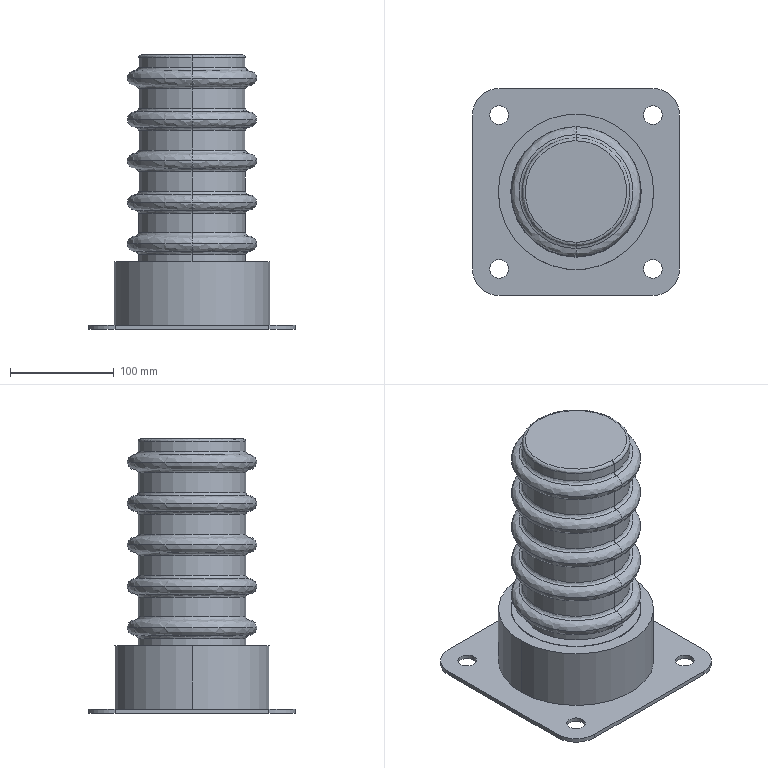Part | STEP file | 921272175 | 2 solids | 83 faces | box 200 x 200 x 265 mm | volume 3161533 mm3 | spline 42 | cylinder 30 | plane 11 | commonest cylinder face diameters 104 x12 18 x8 51.508 x4 125 x2 126 x2 150 x2